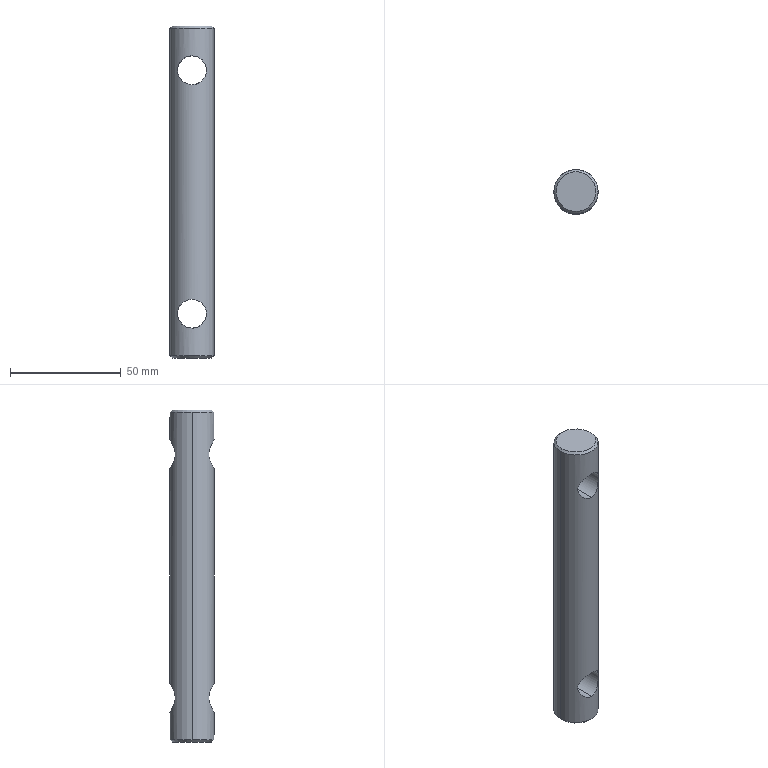Part | STEP file | 1 solid | 12 faces | box 20 x 20 x 150 mm | volume 42054 mm3 | cylinder 6 | cone 4 | plane 2 | commonest cylinder face diameters 13 x4 20 x2